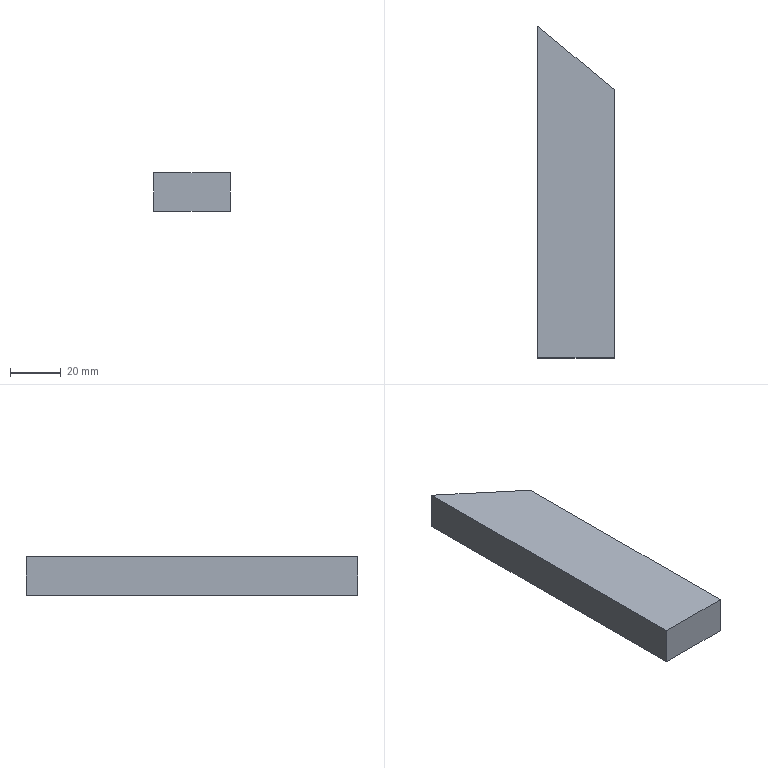Part | NX | features solid 2 | 1 solid | 6 faces | box 30 x 130.944 x 15 mm | volume 53261 mm3 | plane 6
STEP:
#1=CARTESIAN_POINT('',(-150.017,-239.139,0.));
#2=VERTEX_POINT('',#1);
#3=CARTESIAN_POINT('',(-180.017,-239.139,0.));
#4=VERTEX_POINT('',#3);
#5=CARTESIAN_POINT('',(-150.017,-239.139,0.));
#6=DIRECTION('',(1.,0.,0.));
#7=VECTOR('',#6,1000.);
#8=LINE('',#5,#7);
#9=EDGE_CURVE('',#2,#4,#8,.F.);
#10=ORIENTED_EDGE('',*,*,#9,.T.);
#11=CARTESIAN_POINT('',(-180.017,-108.195,0.));
#12=VERTEX_POINT('',#11);
#13=CARTESIAN_POINT('',(-180.017,-164.139,0.));
#14=DIRECTION('',(0.,1.,0.));
#15=VECTOR('',#14,1000.);
#16=LINE('',#13,#15);
#17=EDGE_CURVE('',#4,#12,#16,.T.);
#18=ORIENTED_EDGE('',*,*,#17,.T.);
#19=CARTESIAN_POINT('',(-150.017,-133.368,0.));
#20=VERTEX_POINT('',#19);
#21=CARTESIAN_POINT('',(-274.791,-28.67,0.));
#22=DIRECTION('',(0.766,-0.6428,0.));
#23=VECTOR('',#22,1000.);
#24=LINE('',#21,#23);
#25=EDGE_CURVE('',#20,#12,#24,.F.);
#26=ORIENTED_EDGE('',*,*,#25,.F.);
#27=CARTESIAN_POINT('',(-150.017,-164.139,0.));
#28=DIRECTION('',(0.,1.,0.));
#29=VECTOR('',#28,1000.);
#30=LINE('',#27,#29);
#31=EDGE_CURVE('',#2,#20,#30,.T.);
#32=ORIENTED_EDGE('',*,*,#31,.F.);
#33=EDGE_LOOP('',(#10,#18,#26,#32));
#34=FACE_BOUND('',#33,.T.);
#35=CARTESIAN_POINT('',(-150.017,-164.139,0.));
#36=DIRECTION('',(0.,0.,-1.));
#37=DIRECTION('',(0.,1.,0.));
#38=AXIS2_PLACEMENT_3D('',#35,#36,#37);
#39=PLANE('',#38);
#40=ADVANCED_FACE('',(#34),#39,.T.);
#41=ORIENTED_EDGE('',*,*,#25,.T.);
#42=CARTESIAN_POINT('',(-180.017,-108.195,15.));
#43=VERTEX_POINT('',#42);
#44=CARTESIAN_POINT('',(-180.017,-108.195,-15.));
#45=DIRECTION('',(0.,0.,1.));
#46=VECTOR('',#45,1000.);
#47=LINE('',#44,#46);
#48=EDGE_CURVE('',#12,#43,#47,.T.);
#49=ORIENTED_EDGE('',*,*,#48,.T.);
#50=CARTESIAN_POINT('',(-150.017,-133.368,15.));
#51=VERTEX_POINT('',#50);
#52=CARTESIAN_POINT('',(-134.865,-146.082,15.));
#53=DIRECTION('',(-0.766,0.6428,0.));
#54=VECTOR('',#53,1000.);
#55=LINE('',#52,#54);
#56=EDGE_CURVE('',#51,#43,#55,.T.);
#57=ORIENTED_EDGE('',*,*,#56,.F.);
#58=CARTESIAN_POINT('',(-150.017,-133.368,-15.));
#59=DIRECTION('',(0.,0.,1.));
#60=VECTOR('',#59,1000.);
#61=LINE('',#58,#60);
#62=EDGE_CURVE('',#20,#51,#61,.T.);
#63=ORIENTED_EDGE('',*,*,#62,.F.);
#64=EDGE_LOOP('',(#41,#49,#57,#63));
#65=FACE_BOUND('',#64,.T.);
#66=CARTESIAN_POINT('',(-274.791,-28.67,-15.));
#67=DIRECTION('',(-0.6428,-0.766,0.));
#68=DIRECTION('',(0.766,-0.6428,0.));
#69=AXIS2_PLACEMENT_3D('',#66,#67,#68);
#70=PLANE('',#69);
#71=ADVANCED_FACE('',(#65),#70,.F.);
#72=ORIENTED_EDGE('',*,*,#56,.T.);
#73=CARTESIAN_POINT('',(-180.017,-239.139,15.));
#74=VERTEX_POINT('',#73);
#75=CARTESIAN_POINT('',(-180.017,-164.139,15.));
#76=DIRECTION('',(0.,1.,0.));
#77=VECTOR('',#76,1000.);
#78=LINE('',#75,#77);
#79=EDGE_CURVE('',#74,#43,#78,.T.);
#80=ORIENTED_EDGE('',*,*,#79,.F.);
#81=CARTESIAN_POINT('',(-150.017,-239.139,15.));
#82=VERTEX_POINT('',#81);
#83=CARTESIAN_POINT('',(-150.017,-239.139,15.));
#84=DIRECTION('',(-1.,0.,0.));
#85=VECTOR('',#84,1000.);
#86=LINE('',#83,#85);
#87=EDGE_CURVE('',#82,#74,#86,.T.);
#88=ORIENTED_EDGE('',*,*,#87,.F.);
#89=CARTESIAN_POINT('',(-150.017,-164.139,15.));
#90=DIRECTION('',(0.,1.,0.));
#91=VECTOR('',#90,1000.);
#92=LINE('',#89,#91);
#93=EDGE_CURVE('',#82,#51,#92,.T.);
#94=ORIENTED_EDGE('',*,*,#93,.T.);
#95=EDGE_LOOP('',(#72,#80,#88,#94));
#96=FACE_BOUND('',#95,.T.);
#97=CARTESIAN_POINT('',(-150.017,-164.139,15.));
#98=DIRECTION('',(0.,0.,-1.));
#99=DIRECTION('',(0.,1.,0.));
#100=AXIS2_PLACEMENT_3D('',#97,#98,#99);
#101=PLANE('',#100);
#102=ADVANCED_FACE('',(#96),#101,.F.);
#103=CARTESIAN_POINT('',(-150.017,-239.139,0.));
#104=DIRECTION('',(0.,0.,1.));
#105=VECTOR('',#104,1000.);
#106=LINE('',#103,#105);
#107=EDGE_CURVE('',#2,#82,#106,.T.);
#108=ORIENTED_EDGE('',*,*,#107,.T.);
#109=ORIENTED_EDGE('',*,*,#87,.T.);
#110=CARTESIAN_POINT('',(-180.017,-239.139,0.));
#111=DIRECTION('',(0.,0.,1.));
#112=VECTOR('',#111,1000.);
#113=LINE('',#110,#112);
#114=EDGE_CURVE('',#4,#74,#113,.T.);
#115=ORIENTED_EDGE('',*,*,#114,.F.);
#116=ORIENTED_EDGE('',*,*,#9,.F.);
#117=EDGE_LOOP('',(#108,#109,#115,#116));
#118=FACE_BOUND('',#117,.T.);
#119=CARTESIAN_POINT('',(-150.017,-239.139,0.));
#120=DIRECTION('',(0.,1.,0.));
#121=DIRECTION('',(0.,0.,1.));
#122=AXIS2_PLACEMENT_3D('',#119,#120,#121);
#123=PLANE('',#122);
#124=ADVANCED_FACE('',(#118),#123,.F.);
#125=ORIENTED_EDGE('',*,*,#79,.T.);
#126=ORIENTED_EDGE('',*,*,#48,.F.);
#127=ORIENTED_EDGE('',*,*,#17,.F.);
#128=ORIENTED_EDGE('',*,*,#114,.T.);
#129=EDGE_LOOP('',(#125,#126,#127,#128));
#130=FACE_BOUND('',#129,.T.);
#131=CARTESIAN_POINT('',(-180.017,-164.139,0.));
#132=DIRECTION('',(1.,0.,0.));
#133=DIRECTION('',(0.,0.,-1.));
#134=AXIS2_PLACEMENT_3D('',#131,#132,#133);
#135=PLANE('',#134);
#136=ADVANCED_FACE('',(#130),#135,.F.);
#137=ORIENTED_EDGE('',*,*,#93,.F.);
#138=ORIENTED_EDGE('',*,*,#107,.F.);
#139=ORIENTED_EDGE('',*,*,#31,.T.);
#140=ORIENTED_EDGE('',*,*,#62,.T.);
#141=EDGE_LOOP('',(#137,#138,#139,#140));
#142=FACE_BOUND('',#141,.T.);
#143=CARTESIAN_POINT('',(-150.017,-164.139,0.));
#144=DIRECTION('',(1.,0.,0.));
#145=DIRECTION('',(0.,0.,-1.));
#146=AXIS2_PLACEMENT_3D('',#143,#144,#145);
#147=PLANE('',#146);
#148=ADVANCED_FACE('',(#142),#147,.T.);
#149=CLOSED_SHELL('',(#40,#71,#102,#124,#136,#148));
#150=MANIFOLD_SOLID_BREP('',#149);
#151=(LENGTH_UNIT()NAMED_UNIT(*)SI_UNIT(.MILLI.,.METRE.));
#152=UNCERTAINTY_MEASURE_WITH_UNIT(LENGTH_MEASURE(0.00001),#151,'','');
#153=(NAMED_UNIT(*)PLANE_ANGLE_UNIT()SI_UNIT($,.RADIAN.));
#154=(NAMED_UNIT(*)SI_UNIT($,.STERADIAN.)SOLID_ANGLE_UNIT());
#155=(GEOMETRIC_REPRESENTATION_CONTEXT(3)GLOBAL_UNCERTAINTY_ASSIGNED_CONTEXT((#152))GLOBAL_UNIT_ASSIGNED_CONTEXT((#151,#153,#154))REPRESENTATION_CONTEXT('',''));
#156=ADVANCED_BREP_SHAPE_REPRESENTATION('',(#150),#155);